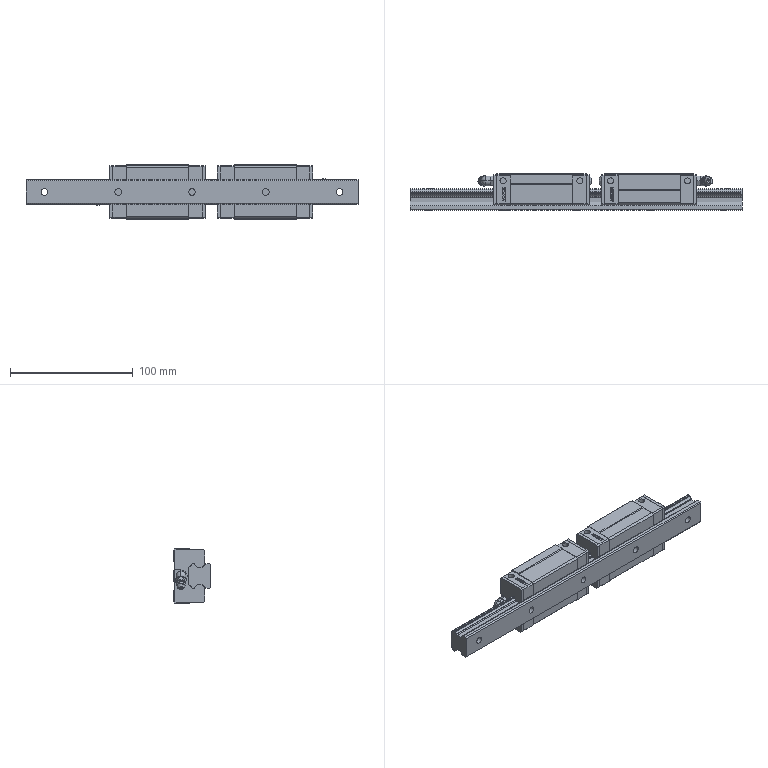Part | SolidWorks | 15 solids | 1579 faces | box 270 x 30 x 44 mm | volume 212143 mm3 | plane 991 | cylinder 466 | cone 92 | spline 12 | sphere 12 | torus 6 | commonest cylinder face diameters 1 x148 0.2 x68 2 x54 4.06 x44 0.1 x36 6 x24